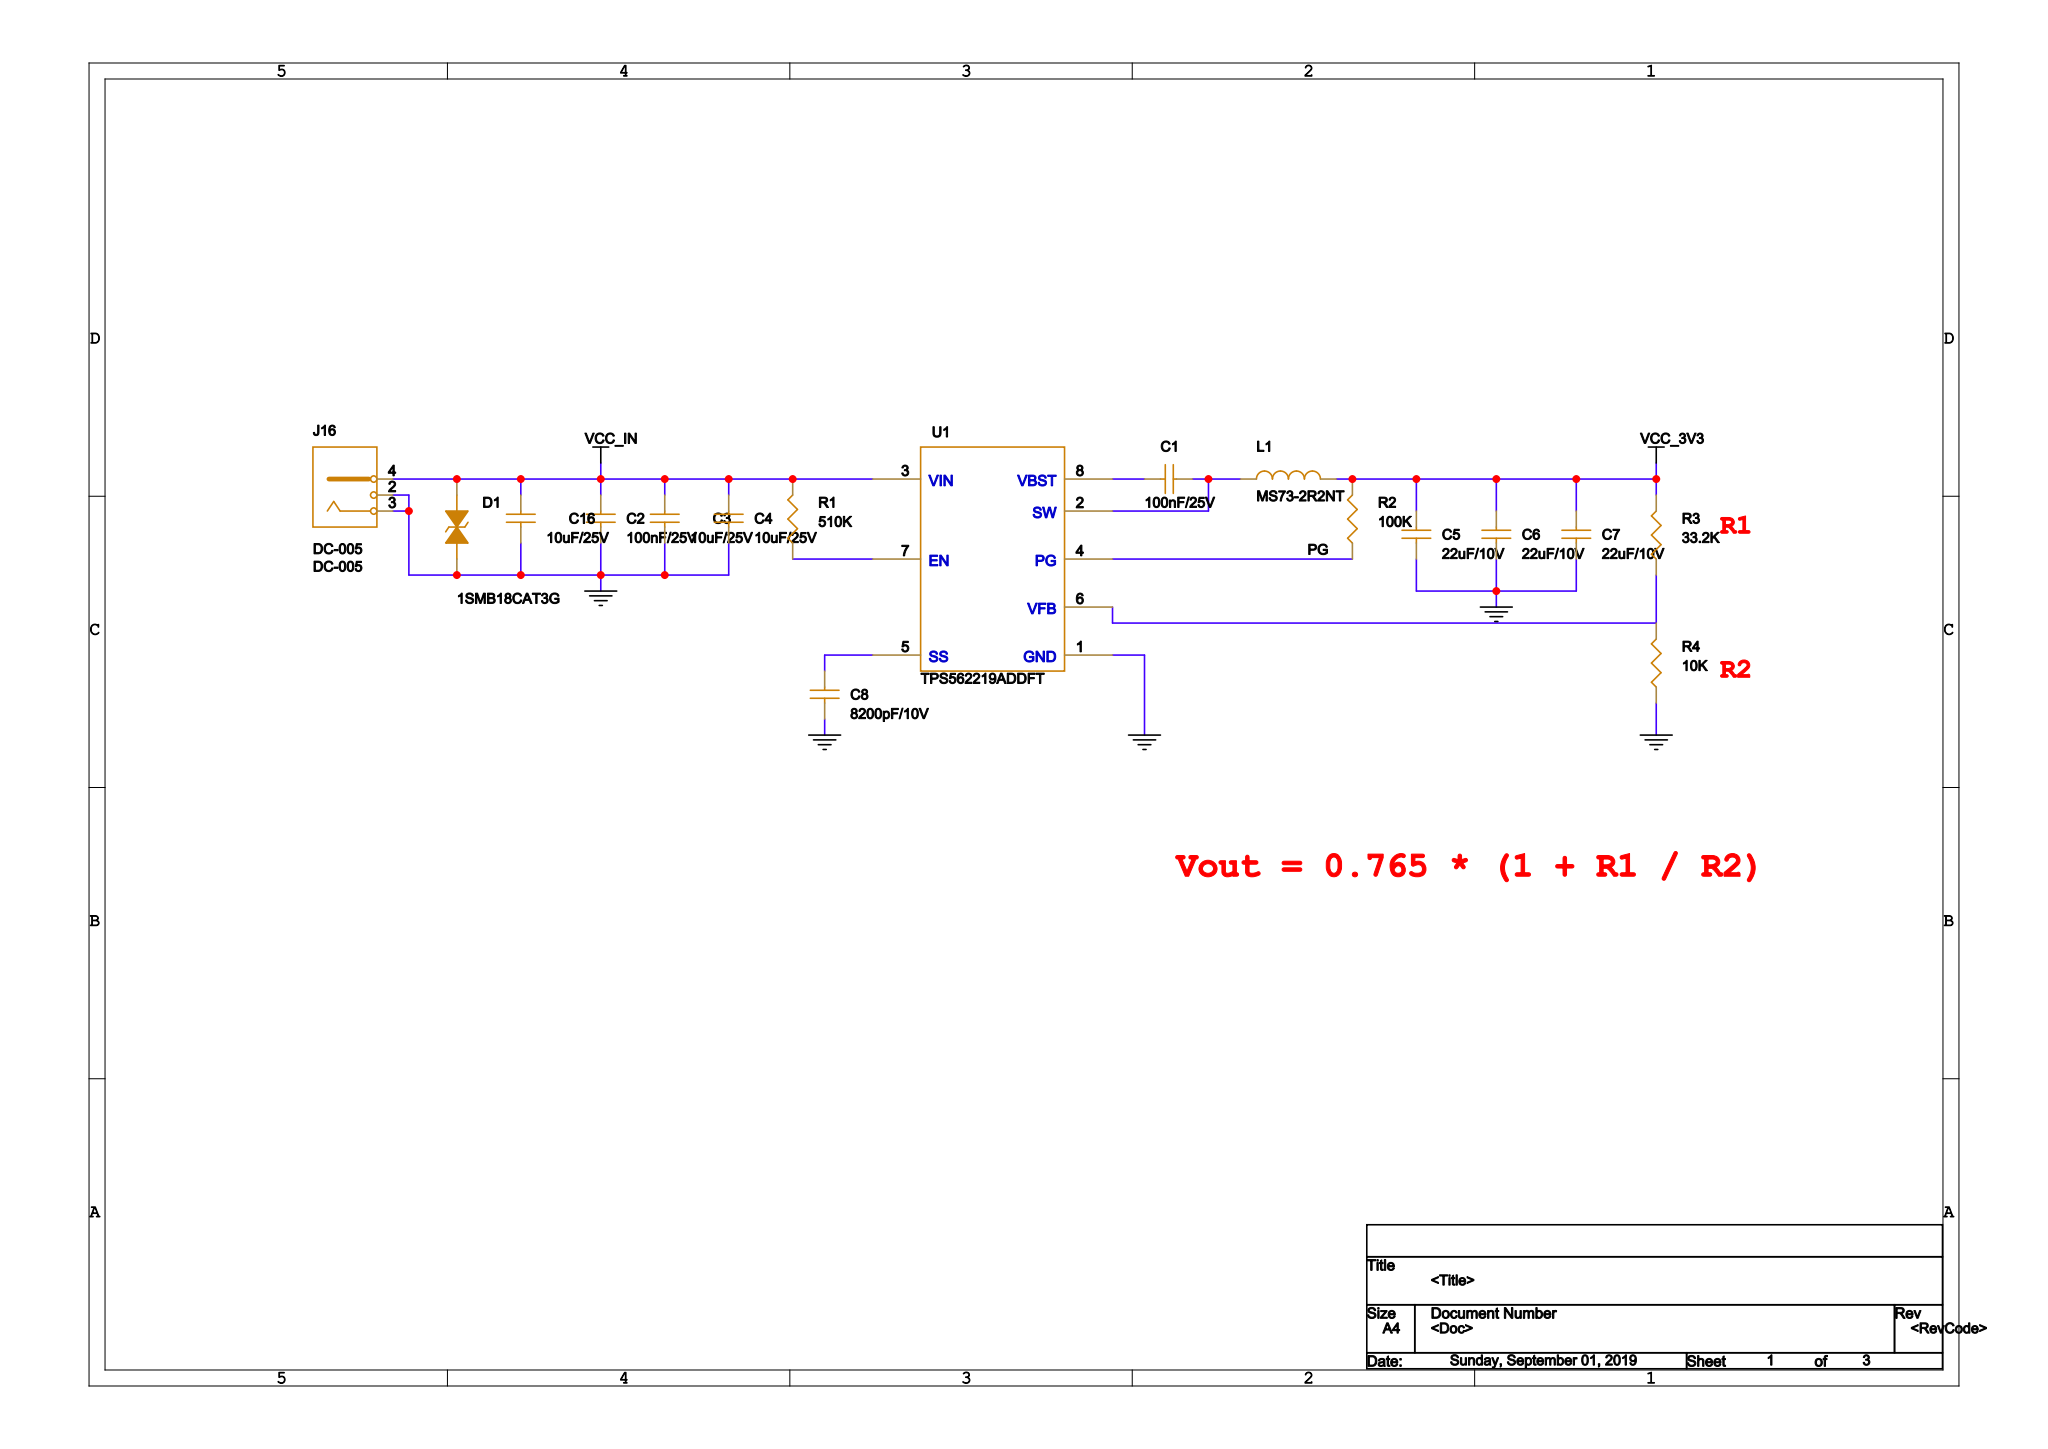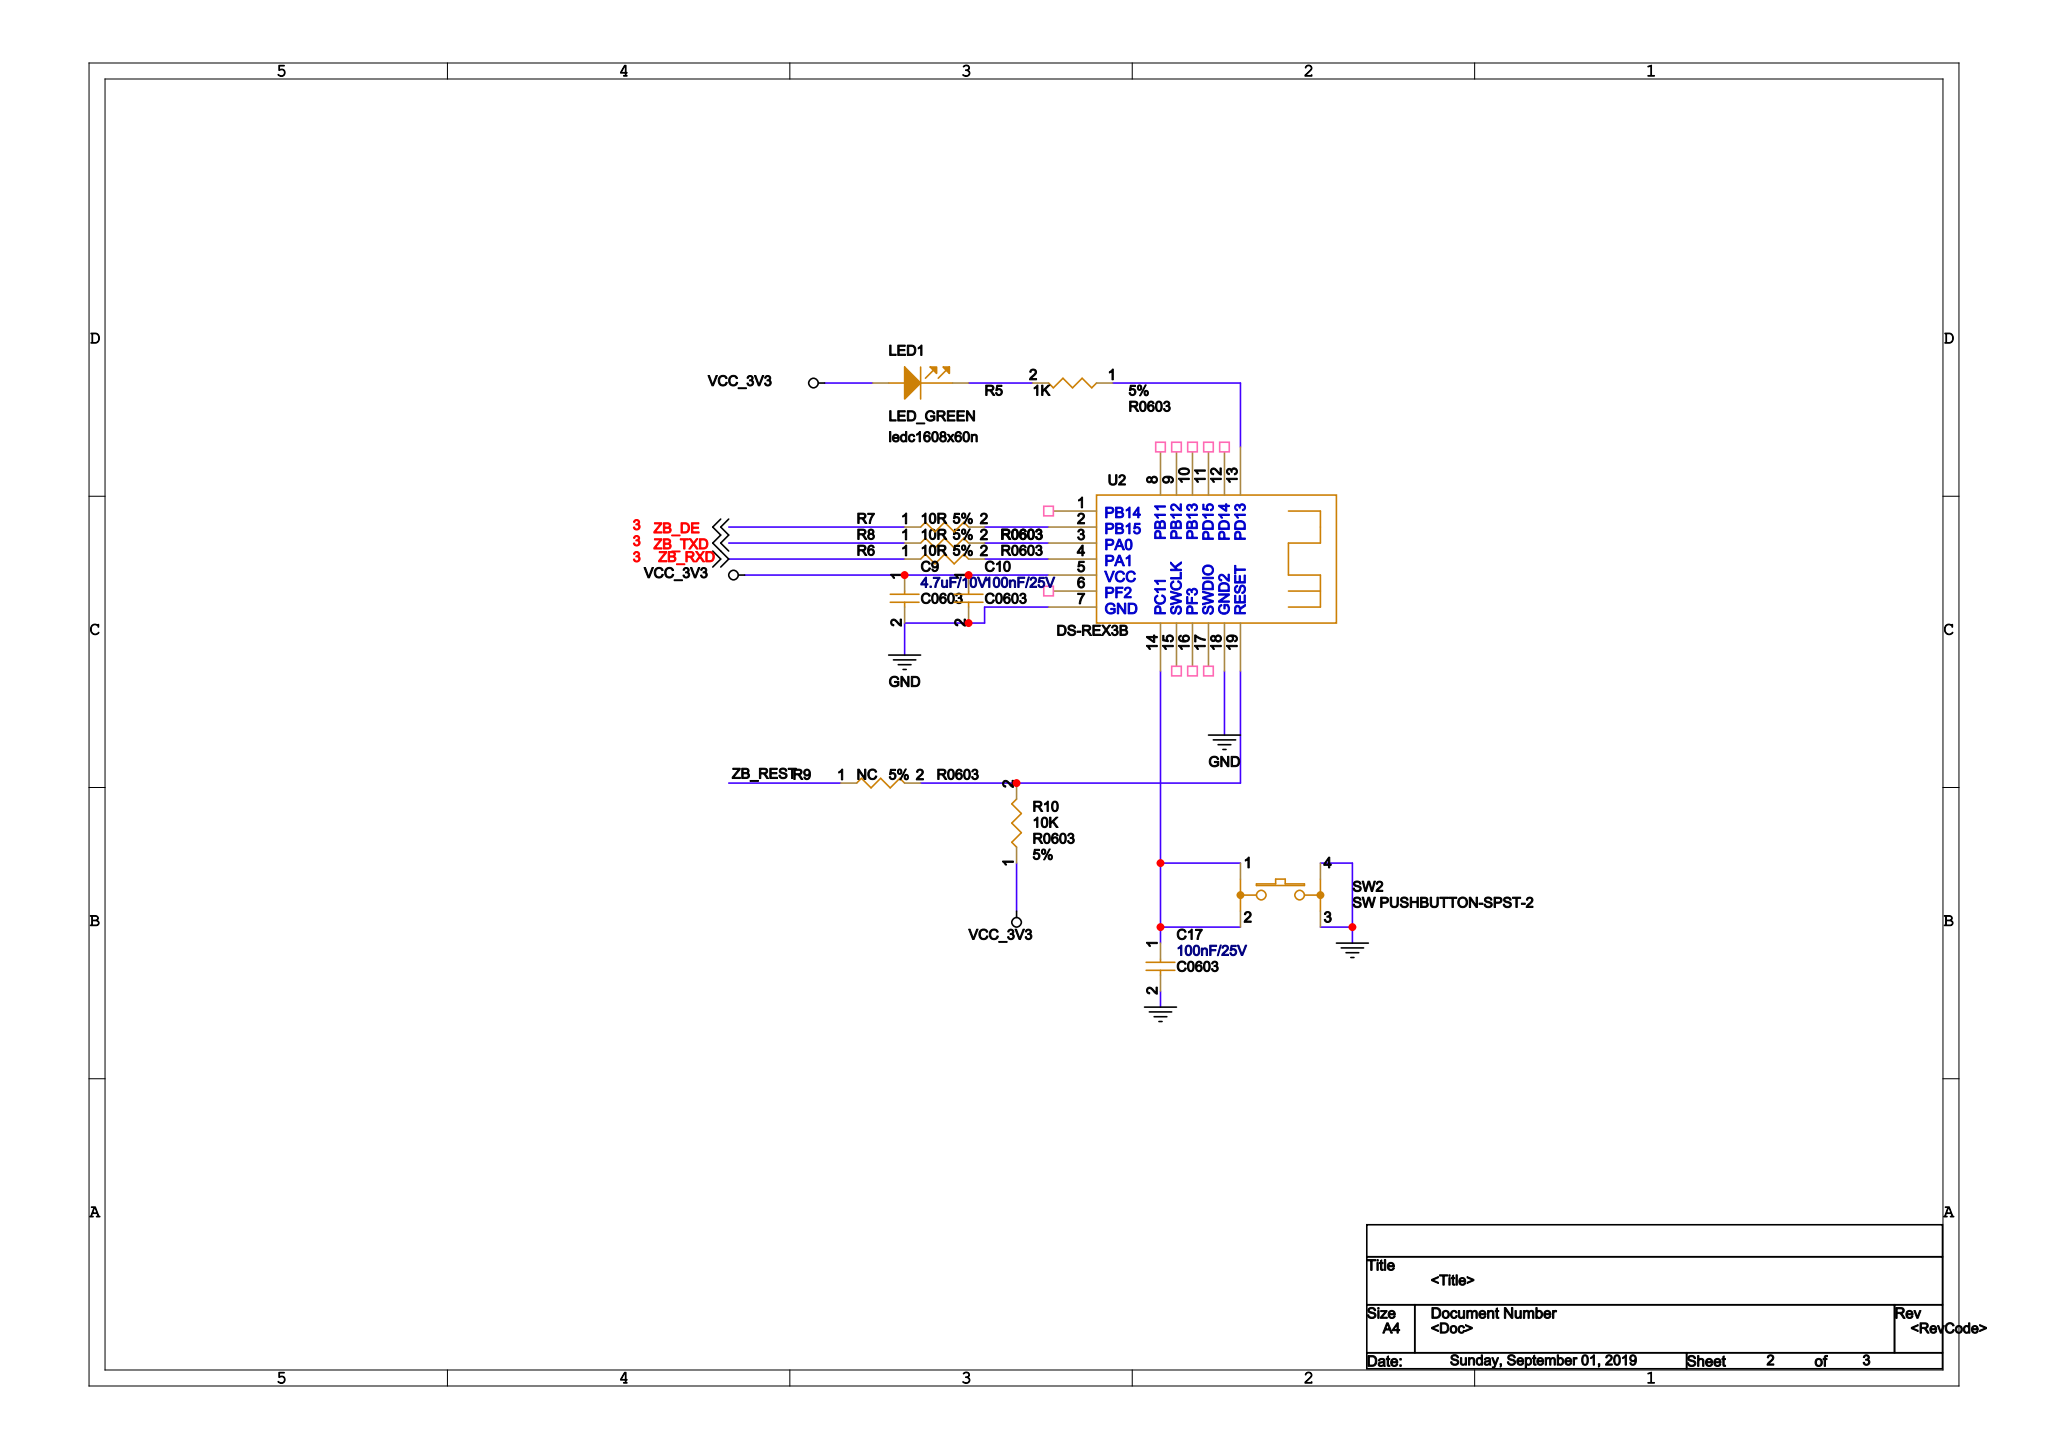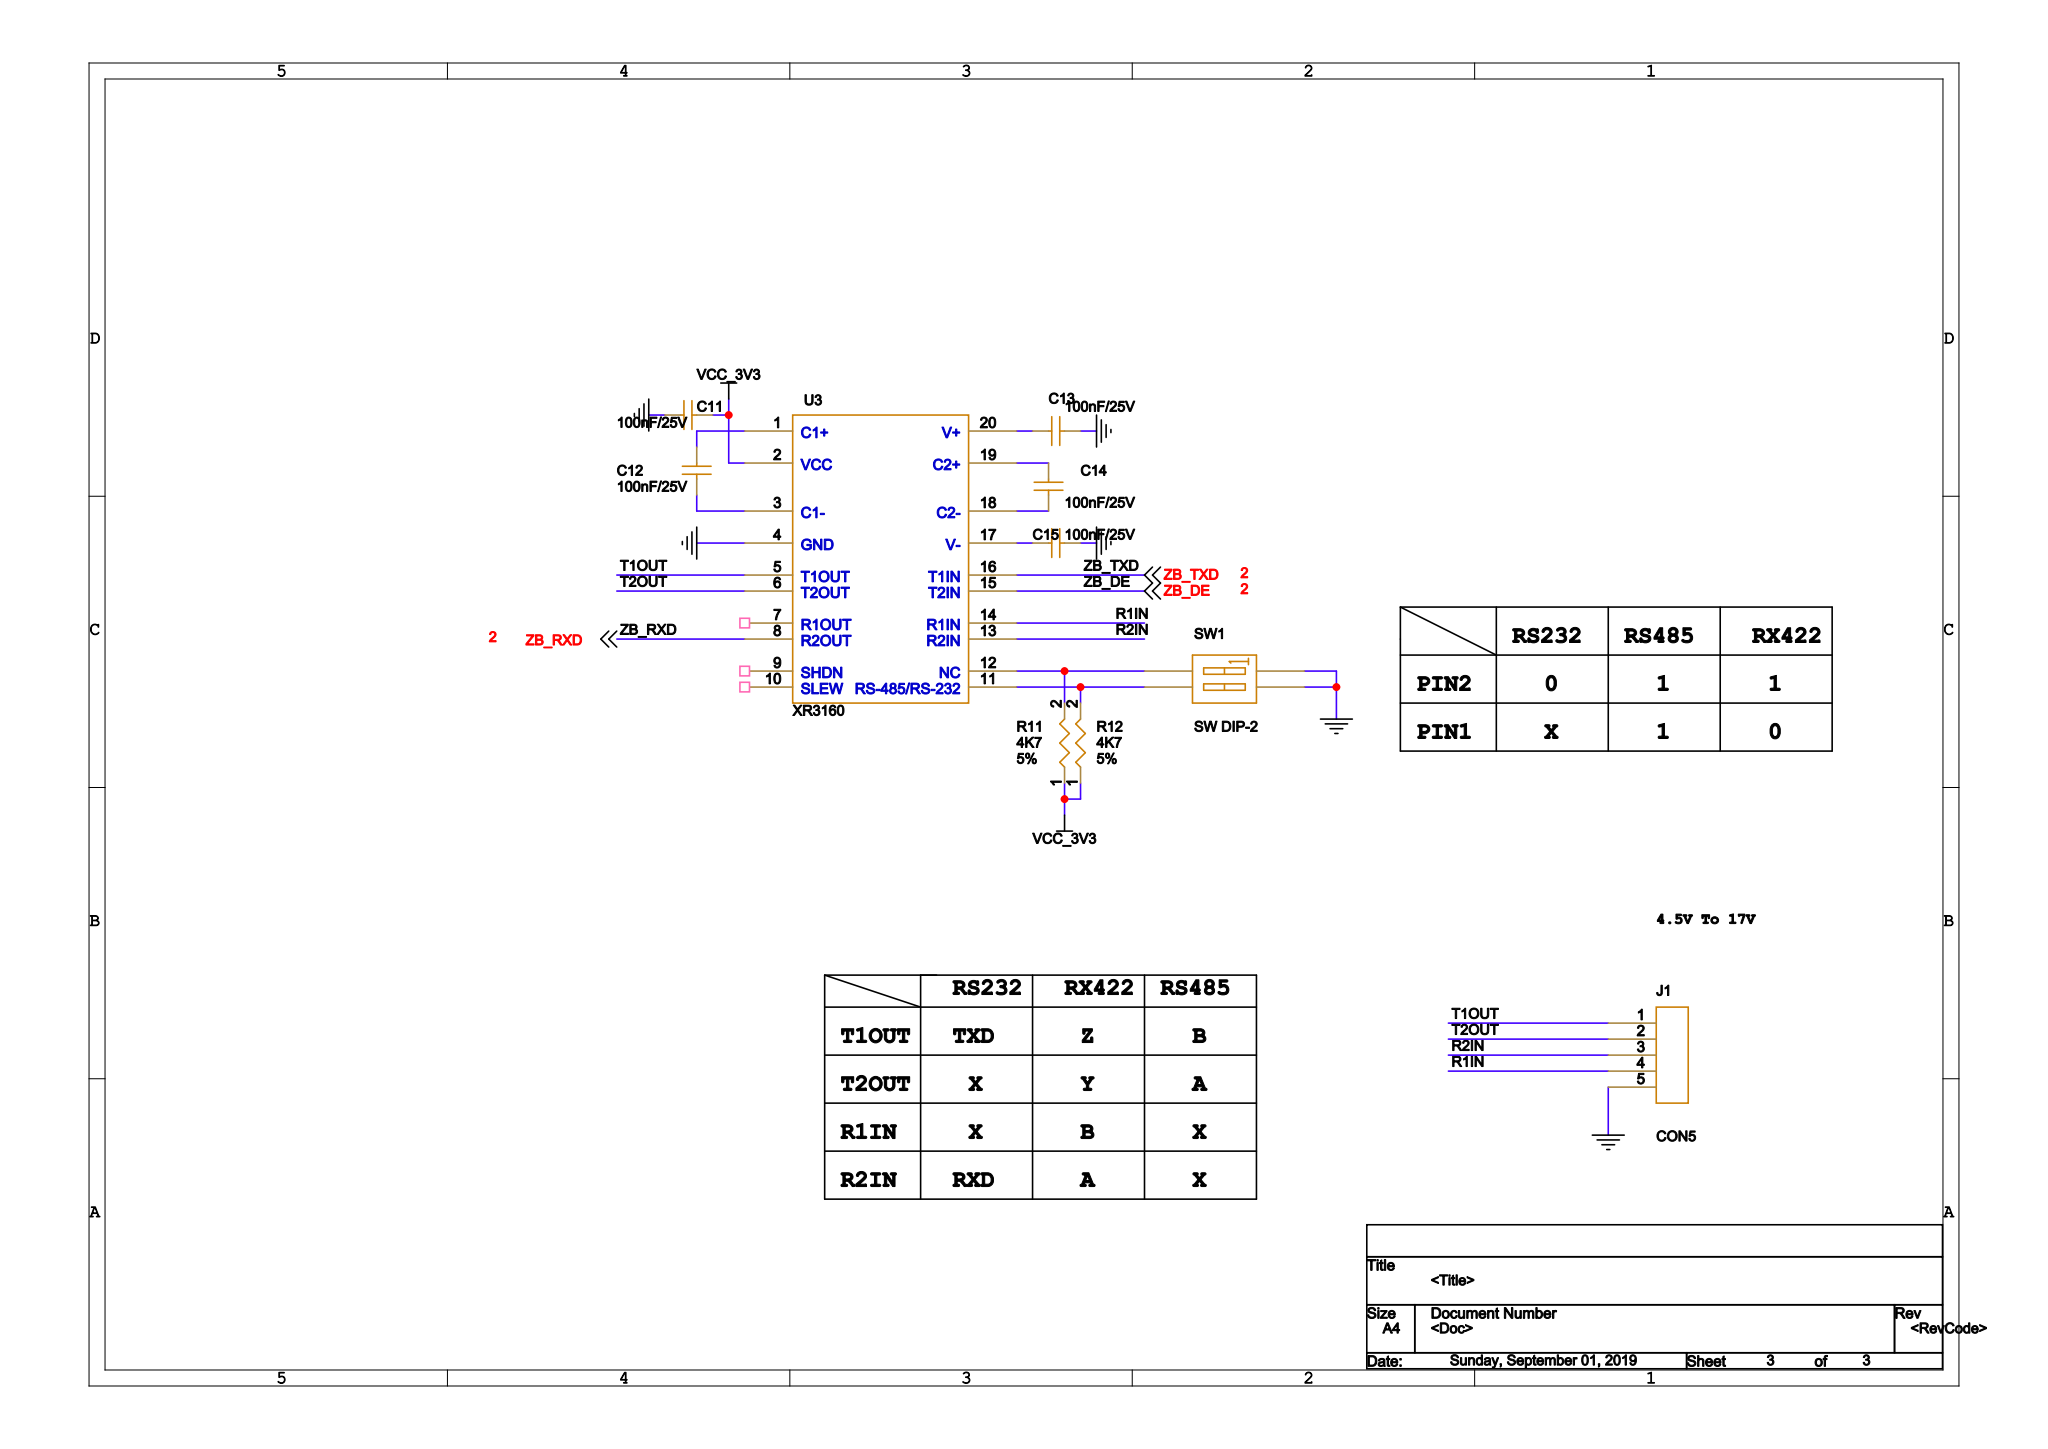Circuit board | Cadence Allegro | 39 parts | 32 nets
Bill of materials:
SYM_NAME,COMP_DEVICE_TYPE,COMP_VALUE,COMP_TOL,COMP_CLASS,REFDES
C0603,CAP NP_C0603_100NF/25V,100nF/25V,,IC,C1
C0603,CAP NP_C0603_100NF/25V,100nF/25V,,IC,C2
C0603,CAP NP_C0603_10UF/25V,10uF/25V,,IC,C3
C0603,CAP NP_C0603_10UF/25V,10uF/25V,,IC,C4
C0603,CAP NP_C0603_22UF/10V,22uF/10V,,IC,C5
C0603,CAP NP_C0603_22UF/10V,22uF/10V,,IC,C6
C0603,CAP NP_C0603_22UF/10V,22uF/10V,,IC,C7
C0603,CAP NP_C0603_8200PF/10V,8200pF/10V,,IC,C8
C0603,CAP NP_C0603_4.7UF,4.7uF,,IC,C9
C0603,CAP NP_C0603_100NF,100nF,,IC,C10
C0603,CAP NP_C0603_100NF/25V,100nF/25V,,IC,C11
C0603,CAP NP_C0603_100NF/25V,100nF/25V,,IC,C12
C0603,CAP NP_C0603_100NF/25V,100nF/25V,,IC,C13
C0603,CAP NP_C0603_100NF/25V,100nF/25V,,IC,C14
C0603,CAP NP_C0603_100NF/25V,100nF/25V,,IC,C15
C0603,CAP NP_C0603_10UF/25V,10uF/25V,,IC,C16
C0603,CAP NP_C0603_100NF,100nF,,IC,C17
SMB,DIODE BI-DIR TRIG_SMB_1SMB18CAT,1SMB18CAT3G,,IC,D1
JK2EDGRC-381-5_1,CON6_0_JK2EDGRC-381-5_1_CON6,CON6,,IC,J1
DC-005,DC0116A_1_DC-005_DC-005,DC-005,,IC,J16
SMD7X7,INDUCTOR_SMD7X7_MS73-2R2NT,MS73-2R2NT,,IC,L1
LEDC1608X60N,LED_LEDC1608X60N_LED_GREEN,LED_GREEN,,IC,LED1
R0603,RESISTOR_R0603_510K,510K,,IC,R1
R0603,RESISTOR_R0603_100K,100K,,IC,R2
R0603,RESISTOR_R0603_33.2K,33.2K,,IC,R3
R0603,RESISTOR_R0603_10K,10K,,IC,R4
R0603,RESISTOR_R0603_1K,1K,,IC,R5
R0603,RESISTOR_R0603_10R,10R,,IC,R6
R0603,RESISTOR_R0603_10R,10R,,IC,R7
R0603,RESISTOR_R0603_10R,10R,,IC,R8
R0603,RESISTOR_R0603_NC,NC,,IC,R9
R0603,RESISTOR_R0603_10K,10K,,IC,R10
R0603,RESISTOR_R0603_4K7,4K7,,IC,R11
R0603,RESISTOR_R0603_4K7,4K7,,IC,R12
DA-02,SW DIP-2_0_DA-02_SW DIP-2,SW DIP-2,,IC,SW1
DIP-4,SW PUSHBUTTON-SPST-2_DIP-4_SW P,SW PUSHBUTTON-SPST-2,,IC,SW2
SOT-8,TPS56X219A_SOT-8_TPS562219ADDFT,TPS562219ADDFT,,IC,U1
DS-REX3B,DS-REX3B_DS-REX3B_DS-REX3B,DS-REX3B,,IC,U2
TSSOP-20_1,XR3160_TSSOP-20_1_XR3160,XR3160,,IC,U3
Netlist (net: part-pin ...):
T1OUT: J1-1 U3-5
T2OUT: J1-2 U3-6
R2IN: J1-3 U3-13
R1IN: J1-4 U3-14
GND: C2-2 C3-2 C4-2 C5-2 C6-2 C7-2 C8-2 C9-2 C10-2 C11-1 C13-2 C15-2 C16-2 C17-2 D1-2 J1-5 J16-2 J16-3 R4-1 SW1-2 SW1-4 SW2-3 SW2-4 U1-1 U2-7 U2-18 U3-4
VCC_IN: C2-1 C3-1 C4-1 C16-1 D1-1 J16-4 R1-2 U1-3
N61291: R1-1 U1-7
N60905: C1-1 L1-1 U1-2
N60901: C1-2 U1-8
VCC_3V3: C5-1 C6-1 C7-1 C9-1 C10-1 C11-2 L1-2 LED1-1 R2-2 R3-2 R10-1 R11-1 R12-1 U2-5 U3-2
N16619079: C12-1 U3-1
N16618981: C12-2 U3-3
N16619067: C13-1 U3-20
N16619023: C14-1 U3-19
N16619027: C14-2 U3-18
N16619145: C15-1 U3-17
N16776578: C17-1 SW2-1 SW2-2 U2-14
N61147: C8-1 U1-5
N16617931: LED1-2 R5-2
N16619497: R11-2 SW1-1 U3-12
N16619504: R12-2 SW1-3 U3-11
N61071: R3-1 R4-2 U1-6
N16617927: R5-1 U2-13
ZB_RXD: R6-1 U3-8
N16617775: R6-2 U2-4
ZB_DE: R7-1 U3-15
N16620380: R7-2 U2-2
ZB_TXD: R8-1 U3-16
N16617771: R8-2 U2-3
ZB_REST: R9-1
N16617845: R9-2 R10-2 U2-19
PG: R2-1 U1-4